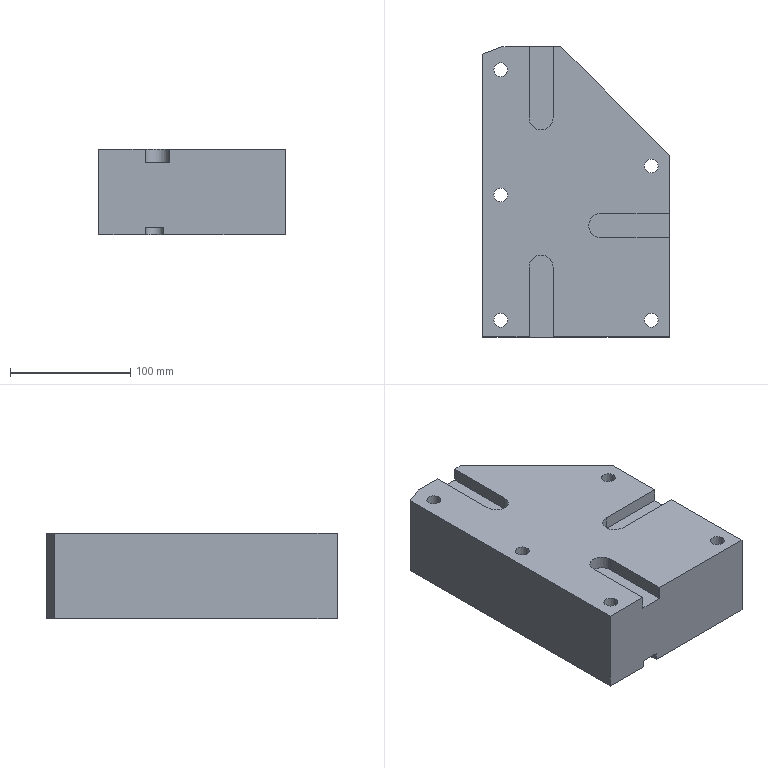Part | NX | features 8 2 | 1 solid | 67 faces | box 155 x 241 x 71 mm | volume 2237140 mm3 | plane 31 | cylinder 28 | cone 8 | commonest cylinder face diameters 20 x7 8.5 x5 11.5 x5 18 x5 5.2 x3 15 x3